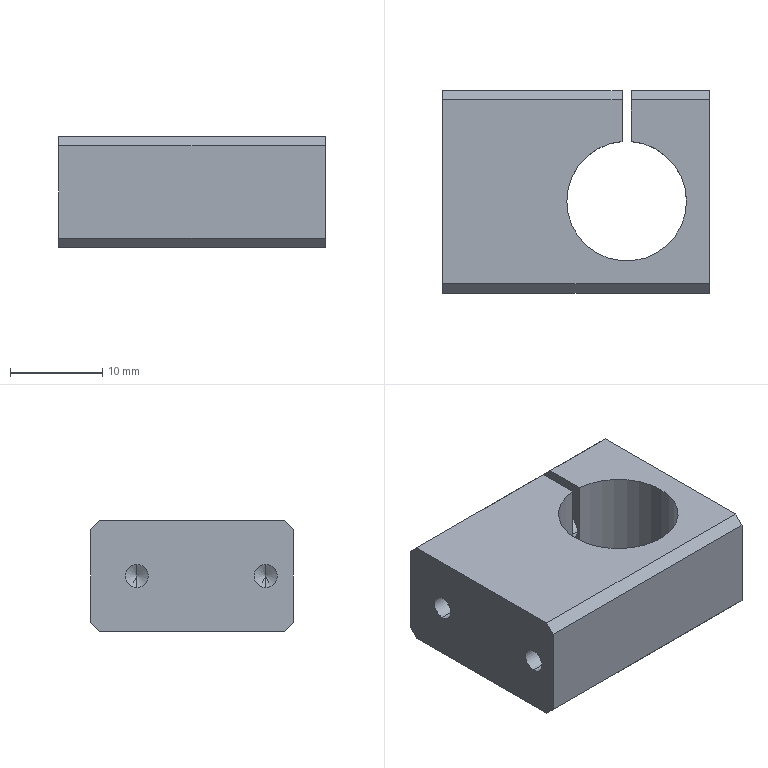NC program | NX | posted with a generic post | part box 29 x 22 x 12 mm
Whole program:
N10 G17 G21 G94 G90
(PLANAR_PROFILE , TOOL : D1)
N12 T20 M6
N14 G54
N16 G17 G0 G90 X-5.5 Y9.5 B0. C0. S9500 M3
N18 G43 Z30. H20
N20 Z0.02
N22 G94 G1 Y6. F850.
N24 Y-6.
N26 Y-9.5
N28 G0 Z-0.06
N30 G1 Y-6.
N32 Y6.
N34 Y9.5
N36 G0 Z-0.14
N38 G1 Y6.
N40 Y-6.
N42 Y-9.5
N44 G0 Z-0.22
N46 G1 Y-6.
N48 Y6.
N50 Y9.5
N52 G0 Z-0.3
N54 G1 Y6.
N56 Y-6.
N58 Y-9.5
N60 G0 Z-0.38
N62 G1 Y-6.
N64 Y6.
N66 Y9.5
N68 G0 Z-0.46
N70 G1 Y6.
N72 Y-6.
N74 Y-9.5
N76 G0 Z-0.54
N78 G1 Y-6.
N80 Y6.
N82 Y9.5
N84 G0 Z-0.62
N86 G1 Y6.
N88 Y-6.
N90 Y-9.5
N92 G0 Z-0.7
N94 G1 Y-6.
N96 Y6.
N98 Y9.5
N100 G0 Z-0.78
N102 G1 Y6.
N104 Y-6.
N106 Y-9.5
N108 G0 Z-0.86
N110 G1 Y-6.
N112 Y6.
N114 Y9.5
N116 G0 Z-0.94
N118 G1 Y6.
N120 Y-6.
N122 Y-9.5
N124 G0 Z-1.02
N126 G1 Y-6.
N128 Y6.
N130 Y9.5
N132 G0 Z-1.1
N134 G1 Y6.
N136 Y-6.
N138 Y-9.5
N140 G0 Z-1.18
N142 G1 Y-6.
N144 Y6.
N146 Y9.5
N148 G0 Z-1.26
N150 G1 Y6.
N152 Y-6.
N154 Y-9.5
N156 G0 Z-1.34
N158 G1 Y-6.
N160 Y6.
N162 Y9.5
N164 G0 Z-1.42
N166 G1 Y6.
N168 Y-6.
N170 Y-9.5
N172 G0 Z-1.5
N174 G1 Y-6.
N176 Y6.
N178 Y9.5
N180 G0 Z-1.58
N182 G1 Y6.
N184 Y-6.
N186 Y-9.5
N188 G0 Z-1.66
N190 G1 Y-6.
N192 Y6.
N194 Y9.5
N196 G0 Z-1.74
N198 G1 Y6.
N200 Y-6.
N202 Y-9.5
N204 G0 Z-1.82
N206 G1 Y-6.
N208 Y6.
N210 Y9.5
N212 G0 Z-1.9
N214 G1 Y6.
N216 Y-6.
N218 Y-9.5
N220 G0 Z-1.98
N222 G1 Y-6.
N224 Y6.
N226 Y9.5
N228 G0 Z-2.06
N230 G1 Y6.
N232 Y-6.
N234 Y-9.5
N236 G0 Z-2.14
N238 G1 Y-6.
N240 Y6.
N242 Y9.5
N244 G0 Z-2.22
N246 G1 Y6.
N248 Y-6.
N250 Y-9.5
N252 G0 Z-2.3
N254 G1 Y-6.
N256 Y6.
N258 Y9.5
N260 G0 Z-2.38
N262 G1 Y6.
N264 Y-6.
N266 Y-9.5
N268 G0 Z-2.46
N270 G1 Y-6.
N272 Y6.
N274 Y9.5
N276 G0 Z-2.54
N278 G1 Y6.
N280 Y-6.
N282 Y-9.5
N284 G0 Z-2.62
N286 G1 Y-6.
N288 Y6.
N290 Y9.5
N292 G0 Z-2.7
N294 G1 Y6.
N296 Y-6.
N298 Y-9.5
N300 G0 Z-2.78
N302 G1 Y-6.
N304 Y6.
N306 Y9.5
N308 G0 Z-2.86
N310 G1 Y6.
N312 Y-6.
N314 Y-9.5
N316 G0 Z-2.94
N318 G1 Y-6.
N320 Y6.
N322 Y9.5
N324 G0 Z-3.02
N326 G1 Y6.
N328 Y-6.
N330 Y-9.5
N332 G0 Z-3.1
N334 G1 Y-6.
N336 Y6.
N338 Y9.5
N340 G0 Z-3.18
N342 G1 Y6.
N344 Y-6.
N346 Y-9.5
N348 G0 Z-3.26
N350 G1 Y-6.
N352 Y6.
N354 Y9.5
N356 G0 Z-3.34
N358 G1 Y6.
N360 Y-6.
N362 Y-9.5
N364 G0 Z-3.42
N366 G1 Y-6.
N368 Y6.
N370 Y9.5
N372 G0 Z-3.5
N374 G1 Y6.
N376 Y-6.
N378 Y-9.5
N380 G0 Z-3.58
N382 G1 Y-6.
N384 Y6.
N386 Y9.5
N388 G0 Z-3.66
N390 G1 Y6.
N392 Y-6.
N394 Y-9.5
N396 G0 Z-3.74
N398 G1 Y-6.
N400 Y6.
N402 Y9.5
N404 G0 Z-3.82
N406 G1 Y6.
N408 Y-6.
N410 Y-9.5
N412 G0 Z-3.9
N414 G1 Y-6.
N416 Y6.
N418 Y9.5
N420 G0 Z-3.98
N422 G1 Y6.
N424 Y-6.
N426 Y-9.5
N428 G0 Z-4.06
N430 G1 Y-6.
N432 Y6.
N434 Y9.5
N436 G0 Z-4.14
N438 G1 Y6.
N440 Y-6.
N442 Y-9.5
N444 G0 Z-4.22
N446 G1 Y-6.
N448 Y6.
N450 Y9.5
N452 G0 Z-4.3
N454 G1 Y6.
N456 Y-6.
N458 Y-9.5
N460 G0 Z-4.38
N462 G1 Y-6.
N464 Y6.
N466 Y9.5
N468 G0 Z-4.46
N470 G1 Y6.
N472 Y-6.
N474 Y-9.5
N476 G0 Z-4.54
N478 G1 Y-6.
N480 Y6.
N482 Y9.5
N484 G0 Z-4.62
N486 G1 Y6.
N488 Y-6.
N490 Y-9.5
N492 G0 Z-4.7
N494 G1 Y-6.
N496 Y6.
N498 Y9.5
N500 G0 Z-4.78
N502 G1 Y6.
N504 Y-6.
N506 Y-9.5
N508 G0 Z-4.86
N510 G1 Y-6.
N512 Y6.
N514 Y9.5
N516 G0 Z-4.94
N518 G1 Y6.
N520 Y-6.
N522 Y-9.5
N524 G0 Z-5.02
N526 G1 Y-6.
N528 Y6.
N530 Y9.5
N532 G0 Z-5.1
N534 G1 Y6.
N536 Y-6.
N538 Y-9.5
N540 G0 Z-5.18
N542 G1 Y-6.
N544 Y6.
N546 Y9.5
N548 G0 Z-5.26
N550 G1 Y6.
N552 Y-6.
N554 Y-9.5
N556 G0 Z-5.34
N558 G1 Y-6.
N560 Y6.
N562 Y9.5
N564 G0 Z-5.42
N566 G1 Y6.
N568 Y-6.
N570 Y-9.5
N572 G0 Z-5.5
N574 G1 Y-6.
N576 Y6.
N578 Y9.5
N580 G0 Z-5.58
N582 G1 Y6.
N584 Y-6.
N586 Y-9.5
N588 G0 Z-5.66
N590 G1 Y-6.
N592 Y6.
N594 Y9.5
N596 G0 Z-5.7
N598 G1 Y6.
N600 Y-6.
N602 Y-9.5
N604 G0 Z30.
N606 M5
N608 M2